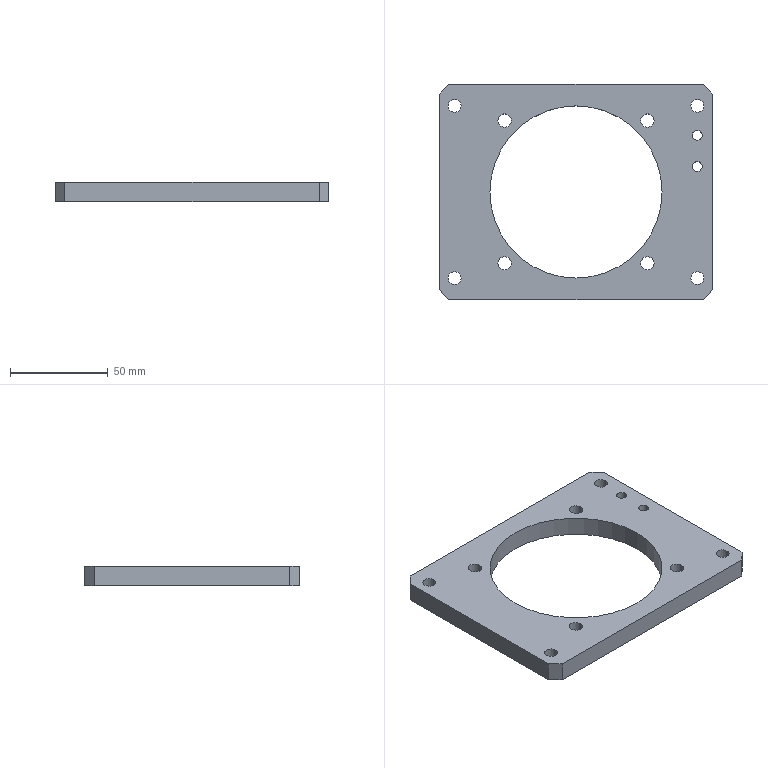Part | SolidWorks | features HoleWzd 2, Chamfer 1, Extrusion 1 | 1 solid | 32 faces | box 140 x 110 x 10 mm | volume 89465 mm3 | cylinder 22 | plane 10 | commonest cylinder face diameters 6.6 x8 6.8 x8 5 x4 88 x2
STEP:
#1=CARTESIAN_POINT('',(65.035,45.511,0.));
#2=VERTEX_POINT('',#1);
#3=CARTESIAN_POINT('',(70.035,45.511,0.));
#4=VERTEX_POINT('',#3);
#5=CARTESIAN_POINT('',(67.535,45.511,0.));
#6=DIRECTION('',(0.,0.,1.));
#7=DIRECTION('',(1.,0.,0.));
#8=AXIS2_PLACEMENT_3D('',#5,#6,#7);
#9=CIRCLE('',#8,2.5);
#10=EDGE_CURVE('',#2,#4,#9,.T.);
#11=ORIENTED_EDGE('',*,*,#10,.F.);
#12=CARTESIAN_POINT('',(65.035,45.511,10.));
#13=VERTEX_POINT('',#12);
#14=CARTESIAN_POINT('',(65.035,45.511,10.));
#15=DIRECTION('',(0.,0.,1.));
#16=VECTOR('',#15,1000.);
#17=LINE('',#14,#16);
#18=EDGE_CURVE('',#2,#13,#17,.T.);
#19=ORIENTED_EDGE('',*,*,#18,.T.);
#20=CARTESIAN_POINT('',(70.035,45.511,10.));
#21=VERTEX_POINT('',#20);
#22=CARTESIAN_POINT('',(67.535,45.511,10.));
#23=DIRECTION('',(0.,0.,1.));
#24=DIRECTION('',(1.,0.,0.));
#25=AXIS2_PLACEMENT_3D('',#22,#23,#24);
#26=CIRCLE('',#25,2.5);
#27=EDGE_CURVE('',#13,#21,#26,.T.);
#28=ORIENTED_EDGE('',*,*,#27,.T.);
#29=CARTESIAN_POINT('',(70.035,45.511,10.));
#30=DIRECTION('',(0.,0.,1.));
#31=VECTOR('',#30,1000.);
#32=LINE('',#29,#31);
#33=EDGE_CURVE('',#4,#21,#32,.T.);
#34=ORIENTED_EDGE('',*,*,#33,.F.);
#35=EDGE_LOOP('',(#11,#19,#28,#34));
#36=FACE_OUTER_BOUND('',#35,.T.);
#37=CARTESIAN_POINT('',(67.535,45.511,10.));
#38=DIRECTION('',(0.,0.,1.));
#39=DIRECTION('',(1.,0.,0.));
#40=AXIS2_PLACEMENT_3D('',#37,#38,#39);
#41=CYLINDRICAL_SURFACE('',#40,2.5);
#42=ADVANCED_FACE('',(#36),#41,.F.);
#43=CARTESIAN_POINT('',(65.035,29.511,0.));
#44=VERTEX_POINT('',#43);
#45=CARTESIAN_POINT('',(70.035,29.511,0.));
#46=VERTEX_POINT('',#45);
#47=CARTESIAN_POINT('',(67.535,29.511,0.));
#48=DIRECTION('',(0.,0.,1.));
#49=DIRECTION('',(1.,0.,0.));
#50=AXIS2_PLACEMENT_3D('',#47,#48,#49);
#51=CIRCLE('',#50,2.5);
#52=EDGE_CURVE('',#44,#46,#51,.T.);
#53=ORIENTED_EDGE('',*,*,#52,.F.);
#54=CARTESIAN_POINT('',(65.035,29.511,10.));
#55=VERTEX_POINT('',#54);
#56=CARTESIAN_POINT('',(65.035,29.511,10.));
#57=DIRECTION('',(0.,0.,1.));
#58=VECTOR('',#57,1000.);
#59=LINE('',#56,#58);
#60=EDGE_CURVE('',#44,#55,#59,.T.);
#61=ORIENTED_EDGE('',*,*,#60,.T.);
#62=CARTESIAN_POINT('',(70.035,29.511,10.));
#63=VERTEX_POINT('',#62);
#64=CARTESIAN_POINT('',(67.535,29.511,10.));
#65=DIRECTION('',(0.,0.,1.));
#66=DIRECTION('',(1.,0.,0.));
#67=AXIS2_PLACEMENT_3D('',#64,#65,#66);
#68=CIRCLE('',#67,2.5);
#69=EDGE_CURVE('',#55,#63,#68,.T.);
#70=ORIENTED_EDGE('',*,*,#69,.T.);
#71=CARTESIAN_POINT('',(70.035,29.511,10.));
#72=DIRECTION('',(0.,0.,1.));
#73=VECTOR('',#72,1000.);
#74=LINE('',#71,#73);
#75=EDGE_CURVE('',#46,#63,#74,.T.);
#76=ORIENTED_EDGE('',*,*,#75,.F.);
#77=EDGE_LOOP('',(#53,#61,#70,#76));
#78=FACE_OUTER_BOUND('',#77,.T.);
#79=CARTESIAN_POINT('',(67.535,29.511,10.));
#80=DIRECTION('',(0.,0.,1.));
#81=DIRECTION('',(1.,0.,0.));
#82=AXIS2_PLACEMENT_3D('',#79,#80,#81);
#83=CYLINDRICAL_SURFACE('',#82,2.5);
#84=ADVANCED_FACE('',(#78),#83,.F.);
#85=CARTESIAN_POINT('',(-34.365,53.011,0.));
#86=VERTEX_POINT('',#85);
#87=CARTESIAN_POINT('',(-27.565,53.011,0.));
#88=VERTEX_POINT('',#87);
#89=CARTESIAN_POINT('',(-30.965,53.011,0.));
#90=DIRECTION('',(0.,0.,1.));
#91=DIRECTION('',(1.,0.,0.));
#92=AXIS2_PLACEMENT_3D('',#89,#90,#91);
#93=CIRCLE('',#92,3.4);
#94=EDGE_CURVE('',#86,#88,#93,.T.);
#95=ORIENTED_EDGE('',*,*,#94,.F.);
#96=CARTESIAN_POINT('',(-34.365,53.011,10.));
#97=VERTEX_POINT('',#96);
#98=CARTESIAN_POINT('',(-34.365,53.011,10.));
#99=DIRECTION('',(0.,0.,1.));
#100=VECTOR('',#99,1000.);
#101=LINE('',#98,#100);
#102=EDGE_CURVE('',#86,#97,#101,.T.);
#103=ORIENTED_EDGE('',*,*,#102,.T.);
#104=CARTESIAN_POINT('',(-27.565,53.011,10.));
#105=VERTEX_POINT('',#104);
#106=CARTESIAN_POINT('',(-30.965,53.011,10.));
#107=DIRECTION('',(0.,0.,1.));
#108=DIRECTION('',(1.,0.,0.));
#109=AXIS2_PLACEMENT_3D('',#106,#107,#108);
#110=CIRCLE('',#109,3.4);
#111=EDGE_CURVE('',#97,#105,#110,.T.);
#112=ORIENTED_EDGE('',*,*,#111,.T.);
#113=CARTESIAN_POINT('',(-27.565,53.011,10.));
#114=DIRECTION('',(0.,0.,1.));
#115=VECTOR('',#114,1000.);
#116=LINE('',#113,#115);
#117=EDGE_CURVE('',#88,#105,#116,.T.);
#118=ORIENTED_EDGE('',*,*,#117,.F.);
#119=EDGE_LOOP('',(#95,#103,#112,#118));
#120=FACE_OUTER_BOUND('',#119,.T.);
#121=CARTESIAN_POINT('',(-30.965,53.011,10.));
#122=DIRECTION('',(0.,0.,1.));
#123=DIRECTION('',(1.,0.,0.));
#124=AXIS2_PLACEMENT_3D('',#121,#122,#123);
#125=CYLINDRICAL_SURFACE('',#124,3.4);
#126=ADVANCED_FACE('',(#120),#125,.F.);
#127=CARTESIAN_POINT('',(38.635,53.011,0.));
#128=VERTEX_POINT('',#127);
#129=CARTESIAN_POINT('',(45.435,53.011,0.));
#130=VERTEX_POINT('',#129);
#131=CARTESIAN_POINT('',(42.035,53.011,0.));
#132=DIRECTION('',(0.,0.,1.));
#133=DIRECTION('',(1.,0.,0.));
#134=AXIS2_PLACEMENT_3D('',#131,#132,#133);
#135=CIRCLE('',#134,3.4);
#136=EDGE_CURVE('',#128,#130,#135,.T.);
#137=ORIENTED_EDGE('',*,*,#136,.F.);
#138=CARTESIAN_POINT('',(38.635,53.011,10.));
#139=VERTEX_POINT('',#138);
#140=CARTESIAN_POINT('',(38.635,53.011,10.));
#141=DIRECTION('',(0.,0.,1.));
#142=VECTOR('',#141,1000.);
#143=LINE('',#140,#142);
#144=EDGE_CURVE('',#128,#139,#143,.T.);
#145=ORIENTED_EDGE('',*,*,#144,.T.);
#146=CARTESIAN_POINT('',(45.435,53.011,10.));
#147=VERTEX_POINT('',#146);
#148=CARTESIAN_POINT('',(42.035,53.011,10.));
#149=DIRECTION('',(0.,0.,1.));
#150=DIRECTION('',(1.,0.,0.));
#151=AXIS2_PLACEMENT_3D('',#148,#149,#150);
#152=CIRCLE('',#151,3.4);
#153=EDGE_CURVE('',#139,#147,#152,.T.);
#154=ORIENTED_EDGE('',*,*,#153,.T.);
#155=CARTESIAN_POINT('',(45.435,53.011,10.));
#156=DIRECTION('',(0.,0.,1.));
#157=VECTOR('',#156,1000.);
#158=LINE('',#155,#157);
#159=EDGE_CURVE('',#130,#147,#158,.T.);
#160=ORIENTED_EDGE('',*,*,#159,.F.);
#161=EDGE_LOOP('',(#137,#145,#154,#160));
#162=FACE_OUTER_BOUND('',#161,.T.);
#163=CARTESIAN_POINT('',(42.035,53.011,10.));
#164=DIRECTION('',(0.,0.,1.));
#165=DIRECTION('',(1.,0.,0.));
#166=AXIS2_PLACEMENT_3D('',#163,#164,#165);
#167=CYLINDRICAL_SURFACE('',#166,3.4);
#168=ADVANCED_FACE('',(#162),#167,.F.);
#169=CARTESIAN_POINT('',(38.635,-19.989,0.));
#170=VERTEX_POINT('',#169);
#171=CARTESIAN_POINT('',(45.435,-19.989,0.));
#172=VERTEX_POINT('',#171);
#173=CARTESIAN_POINT('',(42.035,-19.989,0.));
#174=DIRECTION('',(0.,0.,1.));
#175=DIRECTION('',(1.,0.,0.));
#176=AXIS2_PLACEMENT_3D('',#173,#174,#175);
#177=CIRCLE('',#176,3.4);
#178=EDGE_CURVE('',#170,#172,#177,.T.);
#179=ORIENTED_EDGE('',*,*,#178,.F.);
#180=CARTESIAN_POINT('',(38.635,-19.989,10.));
#181=VERTEX_POINT('',#180);
#182=CARTESIAN_POINT('',(38.635,-19.989,10.));
#183=DIRECTION('',(0.,0.,1.));
#184=VECTOR('',#183,1000.);
#185=LINE('',#182,#184);
#186=EDGE_CURVE('',#170,#181,#185,.T.);
#187=ORIENTED_EDGE('',*,*,#186,.T.);
#188=CARTESIAN_POINT('',(45.435,-19.989,10.));
#189=VERTEX_POINT('',#188);
#190=CARTESIAN_POINT('',(42.035,-19.989,10.));
#191=DIRECTION('',(0.,0.,1.));
#192=DIRECTION('',(1.,0.,0.));
#193=AXIS2_PLACEMENT_3D('',#190,#191,#192);
#194=CIRCLE('',#193,3.4);
#195=EDGE_CURVE('',#181,#189,#194,.T.);
#196=ORIENTED_EDGE('',*,*,#195,.T.);
#197=CARTESIAN_POINT('',(45.435,-19.989,10.));
#198=DIRECTION('',(0.,0.,1.));
#199=VECTOR('',#198,1000.);
#200=LINE('',#197,#199);
#201=EDGE_CURVE('',#172,#189,#200,.T.);
#202=ORIENTED_EDGE('',*,*,#201,.F.);
#203=EDGE_LOOP('',(#179,#187,#196,#202));
#204=FACE_OUTER_BOUND('',#203,.T.);
#205=CARTESIAN_POINT('',(42.035,-19.989,10.));
#206=DIRECTION('',(0.,0.,1.));
#207=DIRECTION('',(1.,0.,0.));
#208=AXIS2_PLACEMENT_3D('',#205,#206,#207);
#209=CYLINDRICAL_SURFACE('',#208,3.4);
#210=ADVANCED_FACE('',(#204),#209,.F.);
#211=CARTESIAN_POINT('',(-34.365,-19.989,0.));
#212=VERTEX_POINT('',#211);
#213=CARTESIAN_POINT('',(-27.565,-19.989,0.));
#214=VERTEX_POINT('',#213);
#215=CARTESIAN_POINT('',(-30.965,-19.989,0.));
#216=DIRECTION('',(0.,0.,1.));
#217=DIRECTION('',(1.,0.,0.));
#218=AXIS2_PLACEMENT_3D('',#215,#216,#217);
#219=CIRCLE('',#218,3.4);
#220=EDGE_CURVE('',#212,#214,#219,.T.);
#221=ORIENTED_EDGE('',*,*,#220,.F.);
#222=CARTESIAN_POINT('',(-34.365,-19.989,10.));
#223=VERTEX_POINT('',#222);
#224=CARTESIAN_POINT('',(-34.365,-19.989,10.));
#225=DIRECTION('',(0.,0.,1.));
#226=VECTOR('',#225,1000.);
#227=LINE('',#224,#226);
#228=EDGE_CURVE('',#212,#223,#227,.T.);
#229=ORIENTED_EDGE('',*,*,#228,.T.);
#230=CARTESIAN_POINT('',(-27.565,-19.989,10.));
#231=VERTEX_POINT('',#230);
#232=CARTESIAN_POINT('',(-30.965,-19.989,10.));
#233=DIRECTION('',(0.,0.,1.));
#234=DIRECTION('',(1.,0.,0.));
#235=AXIS2_PLACEMENT_3D('',#232,#233,#234);
#236=CIRCLE('',#235,3.4);
#237=EDGE_CURVE('',#223,#231,#236,.T.);
#238=ORIENTED_EDGE('',*,*,#237,.T.);
#239=CARTESIAN_POINT('',(-27.565,-19.989,10.));
#240=DIRECTION('',(0.,0.,1.));
#241=VECTOR('',#240,1000.);
#242=LINE('',#239,#241);
#243=EDGE_CURVE('',#214,#231,#242,.T.);
#244=ORIENTED_EDGE('',*,*,#243,.F.);
#245=EDGE_LOOP('',(#221,#229,#238,#244));
#246=FACE_OUTER_BOUND('',#245,.T.);
#247=CARTESIAN_POINT('',(-30.965,-19.989,10.));
#248=DIRECTION('',(0.,0.,1.));
#249=DIRECTION('',(1.,0.,0.));
#250=AXIS2_PLACEMENT_3D('',#247,#248,#249);
#251=CYLINDRICAL_SURFACE('',#250,3.4);
#252=ADVANCED_FACE('',(#246),#251,.F.);
#253=CARTESIAN_POINT('',(64.235,60.511,10.));
#254=VERTEX_POINT('',#253);
#255=CARTESIAN_POINT('',(70.835,60.511,10.));
#256=VERTEX_POINT('',#255);
#257=CARTESIAN_POINT('',(67.535,60.511,10.));
#258=DIRECTION('',(0.,0.,1.));
#259=DIRECTION('',(1.,0.,0.));
#260=AXIS2_PLACEMENT_3D('',#257,#258,#259);
#261=CIRCLE('',#260,3.3);
#262=EDGE_CURVE('',#254,#256,#261,.T.);
#263=ORIENTED_EDGE('',*,*,#262,.T.);
#264=CARTESIAN_POINT('',(70.835,60.511,0.));
#265=VERTEX_POINT('',#264);
#266=CARTESIAN_POINT('',(70.835,60.511,10.));
#267=DIRECTION('',(0.,0.,-1.));
#268=VECTOR('',#267,1000.);
#269=LINE('',#266,#268);
#270=EDGE_CURVE('',#256,#265,#269,.T.);
#271=ORIENTED_EDGE('',*,*,#270,.T.);
#272=CARTESIAN_POINT('',(64.235,60.511,0.));
#273=VERTEX_POINT('',#272);
#274=CARTESIAN_POINT('',(67.535,60.511,0.));
#275=DIRECTION('',(0.,0.,1.));
#276=DIRECTION('',(1.,0.,0.));
#277=AXIS2_PLACEMENT_3D('',#274,#275,#276);
#278=CIRCLE('',#277,3.3);
#279=EDGE_CURVE('',#273,#265,#278,.T.);
#280=ORIENTED_EDGE('',*,*,#279,.F.);
#281=CARTESIAN_POINT('',(64.235,60.511,10.));
#282=DIRECTION('',(0.,0.,-1.));
#283=VECTOR('',#282,1000.);
#284=LINE('',#281,#283);
#285=EDGE_CURVE('',#254,#273,#284,.T.);
#286=ORIENTED_EDGE('',*,*,#285,.F.);
#287=EDGE_LOOP('',(#263,#271,#280,#286));
#288=FACE_OUTER_BOUND('',#287,.T.);
#289=CARTESIAN_POINT('',(67.535,60.511,10.));
#290=DIRECTION('',(0.,0.,-1.));
#291=DIRECTION('',(-1.,0.,0.));
#292=AXIS2_PLACEMENT_3D('',#289,#290,#291);
#293=CYLINDRICAL_SURFACE('',#292,3.3);
#294=ADVANCED_FACE('',(#288),#293,.F.);
#295=CARTESIAN_POINT('',(64.235,-27.489,10.));
#296=VERTEX_POINT('',#295);
#297=CARTESIAN_POINT('',(70.835,-27.489,10.));
#298=VERTEX_POINT('',#297);
#299=CARTESIAN_POINT('',(67.535,-27.489,10.));
#300=DIRECTION('',(0.,0.,1.));
#301=DIRECTION('',(1.,0.,0.));
#302=AXIS2_PLACEMENT_3D('',#299,#300,#301);
#303=CIRCLE('',#302,3.3);
#304=EDGE_CURVE('',#296,#298,#303,.T.);
#305=ORIENTED_EDGE('',*,*,#304,.T.);
#306=CARTESIAN_POINT('',(70.835,-27.489,0.));
#307=VERTEX_POINT('',#306);
#308=CARTESIAN_POINT('',(70.835,-27.489,10.));
#309=DIRECTION('',(0.,0.,-1.));
#310=VECTOR('',#309,1000.);
#311=LINE('',#308,#310);
#312=EDGE_CURVE('',#298,#307,#311,.T.);
#313=ORIENTED_EDGE('',*,*,#312,.T.);
#314=CARTESIAN_POINT('',(64.235,-27.489,0.));
#315=VERTEX_POINT('',#314);
#316=CARTESIAN_POINT('',(67.535,-27.489,0.));
#317=DIRECTION('',(0.,0.,1.));
#318=DIRECTION('',(1.,0.,0.));
#319=AXIS2_PLACEMENT_3D('',#316,#317,#318);
#320=CIRCLE('',#319,3.3);
#321=EDGE_CURVE('',#315,#307,#320,.T.);
#322=ORIENTED_EDGE('',*,*,#321,.F.);
#323=CARTESIAN_POINT('',(64.235,-27.489,10.));
#324=DIRECTION('',(0.,0.,-1.));
#325=VECTOR('',#324,1000.);
#326=LINE('',#323,#325);
#327=EDGE_CURVE('',#296,#315,#326,.T.);
#328=ORIENTED_EDGE('',*,*,#327,.F.);
#329=EDGE_LOOP('',(#305,#313,#322,#328));
#330=FACE_OUTER_BOUND('',#329,.T.);
#331=CARTESIAN_POINT('',(67.535,-27.489,10.));
#332=DIRECTION('',(0.,0.,-1.));
#333=DIRECTION('',(-1.,0.,0.));
#334=AXIS2_PLACEMENT_3D('',#331,#332,#333);
#335=CYLINDRICAL_SURFACE('',#334,3.3);
#336=ADVANCED_FACE('',(#330),#335,.F.);
#337=CARTESIAN_POINT('',(-59.765,-27.489,10.));
#338=VERTEX_POINT('',#337);
#339=CARTESIAN_POINT('',(-53.165,-27.489,10.));
#340=VERTEX_POINT('',#339);
#341=CARTESIAN_POINT('',(-56.465,-27.489,10.));
#342=DIRECTION('',(0.,0.,1.));
#343=DIRECTION('',(1.,0.,0.));
#344=AXIS2_PLACEMENT_3D('',#341,#342,#343);
#345=CIRCLE('',#344,3.3);
#346=EDGE_CURVE('',#338,#340,#345,.T.);
#347=ORIENTED_EDGE('',*,*,#346,.T.);
#348=CARTESIAN_POINT('',(-53.165,-27.489,0.));
#349=VERTEX_POINT('',#348);
#350=CARTESIAN_POINT('',(-53.165,-27.489,10.));
#351=DIRECTION('',(0.,0.,-1.));
#352=VECTOR('',#351,1000.);
#353=LINE('',#350,#352);
#354=EDGE_CURVE('',#340,#349,#353,.T.);
#355=ORIENTED_EDGE('',*,*,#354,.T.);
#356=CARTESIAN_POINT('',(-59.765,-27.489,0.));
#357=VERTEX_POINT('',#356);
#358=CARTESIAN_POINT('',(-56.465,-27.489,0.));
#359=DIRECTION('',(0.,0.,1.));
#360=DIRECTION('',(1.,0.,0.));
#361=AXIS2_PLACEMENT_3D('',#358,#359,#360);
#362=CIRCLE('',#361,3.3);
#363=EDGE_CURVE('',#357,#349,#362,.T.);
#364=ORIENTED_EDGE('',*,*,#363,.F.);
#365=CARTESIAN_POINT('',(-59.765,-27.489,10.));
#366=DIRECTION('',(0.,0.,-1.));
#367=VECTOR('',#366,1000.);
#368=LINE('',#365,#367);
#369=EDGE_CURVE('',#338,#357,#368,.T.);
#370=ORIENTED_EDGE('',*,*,#369,.F.);
#371=EDGE_LOOP('',(#347,#355,#364,#370));
#372=FACE_OUTER_BOUND('',#371,.T.);
#373=CARTESIAN_POINT('',(-56.465,-27.489,10.));
#374=DIRECTION('',(0.,0.,-1.));
#375=DIRECTION('',(-1.,0.,0.));
#376=AXIS2_PLACEMENT_3D('',#373,#374,#375);
#377=CYLINDRICAL_SURFACE('',#376,3.3);
#378=ADVANCED_FACE('',(#372),#377,.F.);
#379=CARTESIAN_POINT('',(-59.765,60.511,10.));
#380=VERTEX_POINT('',#379);
#381=CARTESIAN_POINT('',(-53.165,60.511,10.));
#382=VERTEX_POINT('',#381);
#383=CARTESIAN_POINT('',(-56.465,60.511,10.));
#384=DIRECTION('',(0.,0.,1.));
#385=DIRECTION('',(1.,0.,0.));
#386=AXIS2_PLACEMENT_3D('',#383,#384,#385);
#387=CIRCLE('',#386,3.3);
#388=EDGE_CURVE('',#380,#382,#387,.T.);
#389=ORIENTED_EDGE('',*,*,#388,.T.);
#390=CARTESIAN_POINT('',(-53.165,60.511,0.));
#391=VERTEX_POINT('',#390);
#392=CARTESIAN_POINT('',(-53.165,60.511,10.));
#393=DIRECTION('',(0.,0.,-1.));
#394=VECTOR('',#393,1000.);
#395=LINE('',#392,#394);
#396=EDGE_CURVE('',#382,#391,#395,.T.);
#397=ORIENTED_EDGE('',*,*,#396,.T.);
#398=CARTESIAN_POINT('',(-59.765,60.511,0.));
#399=VERTEX_POINT('',#398);
#400=CARTESIAN_POINT('',(-56.465,60.511,0.));
#401=DIRECTION('',(0.,0.,1.));
#402=DIRECTION('',(1.,0.,0.));
#403=AXIS2_PLACEMENT_3D('',#400,#401,#402);
#404=CIRCLE('',#403,3.3);
#405=EDGE_CURVE('',#399,#391,#404,.T.);
#406=ORIENTED_EDGE('',*,*,#405,.F.);
#407=CARTESIAN_POINT('',(-59.765,60.511,10.));
#408=DIRECTION('',(0.,0.,-1.));
#409=VECTOR('',#408,1000.);
#410=LINE('',#407,#409);
#411=EDGE_CURVE('',#380,#399,#410,.T.);
#412=ORIENTED_EDGE('',*,*,#411,.F.);
#413=EDGE_LOOP('',(#389,#397,#406,#412));
#414=FACE_OUTER_BOUND('',#413,.T.);
#415=CARTESIAN_POINT('',(-56.465,60.511,10.));
#416=DIRECTION('',(0.,0.,-1.));
#417=DIRECTION('',(-1.,0.,0.));
#418=AXIS2_PLACEMENT_3D('',#415,#416,#417);
#419=CYLINDRICAL_SURFACE('',#418,3.3);
#420=ADVANCED_FACE('',(#414),#419,.F.);
#421=CARTESIAN_POINT('',(-38.465,16.511,10.));
#422=VERTEX_POINT('',#421);
#423=CARTESIAN_POINT('',(49.535,16.511,10.));
#424=VERTEX_POINT('',#423);
#425=CARTESIAN_POINT('',(5.535,16.511,10.));
#426=DIRECTION('',(0.,0.,1.));
#427=DIRECTION('',(1.,0.,0.));
#428=AXIS2_PLACEMENT_3D('',#425,#426,#427);
#429=CIRCLE('',#428,44.);
#430=EDGE_CURVE('',#422,#424,#429,.T.);
#431=ORIENTED_EDGE('',*,*,#430,.T.);
#432=CARTESIAN_POINT('',(49.535,16.511,0.));
#433=VERTEX_POINT('',#432);
#434=CARTESIAN_POINT('',(49.535,16.511,10.));
#435=DIRECTION('',(0.,0.,-1.));
#436=VECTOR('',#435,1000.);
#437=LINE('',#434,#436);
#438=EDGE_CURVE('',#424,#433,#437,.T.);
#439=ORIENTED_EDGE('',*,*,#438,.T.);
#440=CARTESIAN_POINT('',(-38.465,16.511,0.));
#441=VERTEX_POINT('',#440);
#442=CARTESIAN_POINT('',(5.535,16.511,0.));
#443=DIRECTION('',(0.,0.,1.));
#444=DIRECTION('',(1.,0.,0.));
#445=AXIS2_PLACEMENT_3D('',#442,#443,#444);
#446=CIRCLE('',#445,44.);
#447=EDGE_CURVE('',#441,#433,#446,.T.);
#448=ORIENTED_EDGE('',*,*,#447,.F.);
#449=CARTESIAN_POINT('',(-38.465,16.511,10.));
#450=DIRECTION('',(0.,0.,-1.));
#451=VECTOR('',#450,1000.);
#452=LINE('',#449,#451);
#453=EDGE_CURVE('',#422,#441,#452,.T.);
#454=ORIENTED_EDGE('',*,*,#453,.F.);
#455=EDGE_LOOP('',(#431,#439,#448,#454));
#456=FACE_OUTER_BOUND('',#455,.T.);
#457=CARTESIAN_POINT('',(5.535,16.511,10.));
#458=DIRECTION('',(0.,0.,-1.));
#459=DIRECTION('',(-1.,0.,0.));
#460=AXIS2_PLACEMENT_3D('',#457,#458,#459);
#461=CYLINDRICAL_SURFACE('',#460,44.);
#462=ADVANCED_FACE('',(#456),#461,.F.);
#463=CARTESIAN_POINT('',(75.535,66.511,10.));
#464=VERTEX_POINT('',#463);
#465=CARTESIAN_POINT('',(75.535,-33.489,10.));
#466=VERTEX_POINT('',#465);
#467=CARTESIAN_POINT('',(75.535,0.,10.));
#468=DIRECTION('',(0.,-1.,0.));
#469=VECTOR('',#468,1000.);
#470=LINE('',#467,#469);
#471=EDGE_CURVE('',#464,#466,#470,.T.);
#472=ORIENTED_EDGE('',*,*,#471,.T.);
#473=CARTESIAN_POINT('',(75.535,-33.489,0.));
#474=VERTEX_POINT('',#473);
#475=CARTESIAN_POINT('',(75.535,-33.489,0.));
#476=DIRECTION('',(0.,0.,-1.));
#477=VECTOR('',#476,1000.);
#478=LINE('',#475,#477);
#479=EDGE_CURVE('',#466,#474,#478,.T.);
#480=ORIENTED_EDGE('',*,*,#479,.T.);
#481=CARTESIAN_POINT('',(75.535,66.511,0.));
#482=VERTEX_POINT('',#481);
#483=CARTESIAN_POINT('',(75.535,0.,0.));
#484=DIRECTION('',(0.,-1.,0.));
#485=VECTOR('',#484,1000.);
#486=LINE('',#483,#485);
#487=EDGE_CURVE('',#482,#474,#486,.T.);
#488=ORIENTED_EDGE('',*,*,#487,.F.);
#489=CARTESIAN_POINT('',(75.535,66.511,10.));
#490=DIRECTION('',(0.,0.,1.));
#491=VECTOR('',#490,1000.);
#492=LINE('',#489,#491);
#493=EDGE_CURVE('',#482,#464,#492,.T.);
#494=ORIENTED_EDGE('',*,*,#493,.T.);
#495=EDGE_LOOP('',(#472,#480,#488,#494));
#496=FACE_OUTER_BOUND('',#495,.T.);
#497=CARTESIAN_POINT('',(75.535,0.,10.));
#498=DIRECTION('',(1.,0.,0.));
#499=DIRECTION('',(0.,1.,0.));
#500=AXIS2_PLACEMENT_3D('',#497,#498,#499);
#501=PLANE('',#500);
#502=ADVANCED_FACE('',(#496),#501,.T.);
#503=CARTESIAN_POINT('',(-59.465,71.511,10.));
#504=VERTEX_POINT('',#503);
#505=CARTESIAN_POINT('',(70.535,71.511,10.));
#506=VERTEX_POINT('',#505);
#507=CARTESIAN_POINT('',(0.,71.511,10.));
#508=DIRECTION('',(1.,0.,0.));
#509=VECTOR('',#508,1000.);
#510=LINE('',#507,#509);
#511=EDGE_CURVE('',#504,#506,#510,.T.);
#512=ORIENTED_EDGE('',*,*,#511,.T.);
#513=CARTESIAN_POINT('',(70.535,71.511,0.));
#514=VERTEX_POINT('',#513);
#515=CARTESIAN_POINT('',(70.535,71.511,10.));
#516=DIRECTION('',(0.,0.,-1.));
#517=VECTOR('',#516,1000.);
#518=LINE('',#515,#517);
#519=EDGE_CURVE('',#506,#514,#518,.T.);
#520=ORIENTED_EDGE('',*,*,#519,.T.);
#521=CARTESIAN_POINT('',(-59.465,71.511,0.));
#522=VERTEX_POINT('',#521);
#523=CARTESIAN_POINT('',(0.,71.511,0.));
#524=DIRECTION('',(1.,0.,0.));
#525=VECTOR('',#524,1000.);
#526=LINE('',#523,#525);
#527=EDGE_CURVE('',#522,#514,#526,.T.);
#528=ORIENTED_EDGE('',*,*,#527,.F.);
#529=CARTESIAN_POINT('',(-59.465,71.511,10.));
#530=DIRECTION('',(0.,0.,1.));
#531=VECTOR('',#530,1000.);
#532=LINE('',#529,#531);
#533=EDGE_CURVE('',#522,#504,#532,.T.);
#534=ORIENTED_EDGE('',*,*,#533,.T.);
#535=EDGE_LOOP('',(#512,#520,#528,#534));
#536=FACE_OUTER_BOUND('',#535,.T.);
#537=CARTESIAN_POINT('',(0.,71.511,10.));
#538=DIRECTION('',(0.,1.,0.));
#539=DIRECTION('',(0.,0.,1.));
#540=AXIS2_PLACEMENT_3D('',#537,#538,#539);
#541=PLANE('',#540);
#542=ADVANCED_FACE('',(#536),#541,.T.);
#543=CARTESIAN_POINT('',(-64.465,66.511,10.));
#544=VERTEX_POINT('',#543);
#545=CARTESIAN_POINT('',(-64.465,-33.489,10.));
#546=VERTEX_POINT('',#545);
#547=CARTESIAN_POINT('',(-64.465,0.,10.));
#548=DIRECTION('',(0.,-1.,0.));
#549=VECTOR('',#548,1000.);
#550=LINE('',#547,#549);
#551=EDGE_CURVE('',#544,#546,#550,.T.);
#552=ORIENTED_EDGE('',*,*,#551,.F.);
#553=CARTESIAN_POINT('',(-64.465,66.511,0.));
#554=VERTEX_POINT('',#553);
#555=CARTESIAN_POINT('',(-64.465,66.511,0.));
#556=DIRECTION('',(0.,0.,-1.));
#557=VECTOR('',#556,1000.);
#558=LINE('',#555,#557);
#559=EDGE_CURVE('',#544,#554,#558,.T.);
#560=ORIENTED_EDGE('',*,*,#559,.T.);
#561=CARTESIAN_POINT('',(-64.465,-33.489,0.));
#562=VERTEX_POINT('',#561);
#563=CARTESIAN_POINT('',(-64.465,0.,0.));
#564=DIRECTION('',(0.,-1.,0.));
#565=VECTOR('',#564,1000.);
#566=LINE('',#563,#565);
#567=EDGE_CURVE('',#554,#562,#566,.T.);
#568=ORIENTED_EDGE('',*,*,#567,.T.);
#569=CARTESIAN_POINT('',(-64.465,-33.489,10.));
#570=DIRECTION('',(0.,0.,1.));
#571=VECTOR('',#570,1000.);
#572=LINE('',#569,#571);
#573=EDGE_CURVE('',#562,#546,#572,.T.);
#574=ORIENTED_EDGE('',*,*,#573,.T.);
#575=EDGE_LOOP('',(#552,#560,#568,#574));
#576=FACE_OUTER_BOUND('',#575,.T.);
#577=CARTESIAN_POINT('',(-64.465,0.,10.));
#578=DIRECTION('',(1.,0.,0.));
#579=DIRECTION('',(0.,0.,-1.));
#580=AXIS2_PLACEMENT_3D('',#577,#578,#579);
#581=PLANE('',#580);
#582=ADVANCED_FACE('',(#576),#581,.F.);
#583=ORIENTED_EDGE('',*,*,#438,.F.);
#584=CARTESIAN_POINT('',(5.535,16.511,10.));
#585=DIRECTION('',(0.,0.,1.));
#586=DIRECTION('',(1.,0.,0.));
#587=AXIS2_PLACEMENT_3D('',#584,#585,#586);
#588=CIRCLE('',#587,44.);
#589=EDGE_CURVE('',#424,#422,#588,.T.);
#590=ORIENTED_EDGE('',*,*,#589,.T.);
#591=ORIENTED_EDGE('',*,*,#453,.T.);
#592=CARTESIAN_POINT('',(5.535,16.511,0.));
#593=DIRECTION('',(0.,0.,1.));
#594=DIRECTION('',(1.,0.,0.));
#595=AXIS2_PLACEMENT_3D('',#592,#593,#594);
#596=CIRCLE('',#595,44.);
#597=EDGE_CURVE('',#433,#441,#596,.T.);
#598=ORIENTED_EDGE('',*,*,#597,.F.);
#599=EDGE_LOOP('',(#583,#590,#591,#598));
#600=FACE_OUTER_BOUND('',#599,.T.);
#601=CARTESIAN_POINT('',(5.535,16.511,10.));
#602=DIRECTION('',(0.,0.,-1.));
#603=DIRECTION('',(-1.,0.,0.));
#604=AXIS2_PLACEMENT_3D('',#601,#602,#603);
#605=CYLINDRICAL_SURFACE('',#604,44.);
#606=ADVANCED_FACE('',(#600),#605,.F.);
#607=ORIENTED_EDGE('',*,*,#396,.F.);
#608=CARTESIAN_POINT('',(-56.465,60.511,10.));
#609=DIRECTION('',(0.,0.,1.));
#610=DIRECTION('',(1.,0.,0.));
#611=AXIS2_PLACEMENT_3D('',#608,#609,#610);
#612=CIRCLE('',#611,3.3);
#613=EDGE_CURVE('',#382,#380,#612,.T.);
#614=ORIENTED_EDGE('',*,*,#613,.T.);
#615=ORIENTED_EDGE('',*,*,#411,.T.);
#616=CARTESIAN_POINT('',(-56.465,60.511,0.));
#617=DIRECTION('',(0.,0.,1.));
#618=DIRECTION('',(1.,0.,0.));
#619=AXIS2_PLACEMENT_3D('',#616,#617,#618);
#620=CIRCLE('',#619,3.3);
#621=EDGE_CURVE('',#391,#399,#620,.T.);
#622=ORIENTED_EDGE('',*,*,#621,.F.);
#623=EDGE_LOOP('',(#607,#614,#615,#622));
#624=FACE_OUTER_BOUND('',#623,.T.);
#625=CARTESIAN_POINT('',(-56.465,60.511,10.));
#626=DIRECTION('',(0.,0.,-1.));
#627=DIRECTION('',(-1.,0.,0.));
#628=AXIS2_PLACEMENT_3D('',#625,#626,#627);
#629=CYLINDRICAL_SURFACE('',#628,3.3);
#630=ADVANCED_FACE('',(#624),#629,.F.);
#631=ORIENTED_EDGE('',*,*,#354,.F.);
#632=CARTESIAN_POINT('',(-56.465,-27.489,10.));
#633=DIRECTION('',(0.,0.,1.));
#634=DIRECTION('',(1.,0.,0.));
#635=AXIS2_PLACEMENT_3D('',#632,#633,#634);
#636=CIRCLE('',#635,3.3);
#637=EDGE_CURVE('',#340,#338,#636,.T.);
#638=ORIENTED_EDGE('',*,*,#637,.T.);
#639=ORIENTED_EDGE('',*,*,#369,.T.);
#640=CARTESIAN_POINT('',(-56.465,-27.489,0.));
#641=DIRECTION('',(0.,0.,1.));
#642=DIRECTION('',(1.,0.,0.));
#643=AXIS2_PLACEMENT_3D('',#640,#641,#642);
#644=CIRCLE('',#643,3.3);
#645=EDGE_CURVE('',#349,#357,#644,.T.);
#646=ORIENTED_EDGE('',*,*,#645,.F.);
#647=EDGE_LOOP('',(#631,#638,#639,#646));
#648=FACE_OUTER_BOUND('',#647,.T.);
#649=CARTESIAN_POINT('',(-56.465,-27.489,10.));
#650=DIRECTION('',(0.,0.,-1.));
#651=DIRECTION('',(-1.,0.,0.));
#652=AXIS2_PLACEMENT_3D('',#649,#650,#651);
#653=CYLINDRICAL_SURFACE('',#652,3.3);
#654=ADVANCED_FACE('',(#648),#653,.F.);
#655=ORIENTED_EDGE('',*,*,#312,.F.);
#656=CARTESIAN_POINT('',(67.535,-27.489,10.));
#657=DIRECTION('',(0.,0.,1.));
#658=DIRECTION('',(1.,0.,0.));
#659=AXIS2_PLACEMENT_3D('',#656,#657,#658);
#660=CIRCLE('',#659,3.3);
#661=EDGE_CURVE('',#298,#296,#660,.T.);
#662=ORIENTED_EDGE('',*,*,#661,.T.);
#663=ORIENTED_EDGE('',*,*,#327,.T.);
#664=CARTESIAN_POINT('',(67.535,-27.489,0.));
#665=DIRECTION('',(0.,0.,1.));
#666=DIRECTION('',(1.,0.,0.));
#667=AXIS2_PLACEMENT_3D('',#664,#665,#666);
#668=CIRCLE('',#667,3.3);
#669=EDGE_CURVE('',#307,#315,#668,.T.);
#670=ORIENTED_EDGE('',*,*,#669,.F.);
#671=EDGE_LOOP('',(#655,#662,#663,#670));
#672=FACE_OUTER_BOUND('',#671,.T.);
#673=CARTESIAN_POINT('',(67.535,-27.489,10.));
#674=DIRECTION('',(0.,0.,-1.));
#675=DIRECTION('',(-1.,0.,0.));
#676=AXIS2_PLACEMENT_3D('',#673,#674,#675);
#677=CYLINDRICAL_SURFACE('',#676,3.3);
#678=ADVANCED_FACE('',(#672),#677,.F.);
#679=ORIENTED_EDGE('',*,*,#270,.F.);
#680=CARTESIAN_POINT('',(67.535,60.511,10.));
#681=DIRECTION('',(0.,0.,1.));
#682=DIRECTION('',(1.,0.,0.));
#683=AXIS2_PLACEMENT_3D('',#680,#681,#682);
#684=CIRCLE('',#683,3.3);
#685=EDGE_CURVE('',#256,#254,#684,.T.);
#686=ORIENTED_EDGE('',*,*,#685,.T.);
#687=ORIENTED_EDGE('',*,*,#285,.T.);
#688=CARTESIAN_POINT('',(67.535,60.511,0.));
#689=DIRECTION('',(0.,0.,1.));
#690=DIRECTION('',(1.,0.,0.));
#691=AXIS2_PLACEMENT_3D('',#688,#689,#690);
#692=CIRCLE('',#691,3.3);
#693=EDGE_CURVE('',#265,#273,#692,.T.);
#694=ORIENTED_EDGE('',*,*,#693,.F.);
#695=EDGE_LOOP('',(#679,#686,#687,#694));
#696=FACE_OUTER_BOUND('',#695,.T.);
#697=CARTESIAN_POINT('',(67.535,60.511,10.));
#698=DIRECTION('',(0.,0.,-1.));
#699=DIRECTION('',(-1.,0.,0.));
#700=AXIS2_PLACEMENT_3D('',#697,#698,#699);
#701=CYLINDRICAL_SURFACE('',#700,3.3);
#702=ADVANCED_FACE('',(#696),#701,.F.);
#703=CARTESIAN_POINT('',(-59.465,-38.489,0.));
#704=VERTEX_POINT('',#703);
#705=CARTESIAN_POINT('',(70.535,-38.489,0.));
#706=VERTEX_POINT('',#705);
#707=CARTESIAN_POINT('',(0.,-38.489,0.));
#708=DIRECTION('',(1.,0.,0.));
#709=VECTOR('',#708,1000.);
#710=LINE('',#707,#709);
#711=EDGE_CURVE('',#704,#706,#710,.T.);
#712=ORIENTED_EDGE('',*,*,#711,.T.);
#713=CARTESIAN_POINT('',(70.535,-38.489,10.));
#714=VERTEX_POINT('',#713);
#715=CARTESIAN_POINT('',(70.535,-38.489,10.));
#716=DIRECTION('',(0.,0.,1.));
#717=VECTOR('',#716,1000.);
#718=LINE('',#715,#717);
#719=EDGE_CURVE('',#706,#714,#718,.T.);
#720=ORIENTED_EDGE('',*,*,#719,.T.);
#721=CARTESIAN_POINT('',(-59.465,-38.489,10.));
#722=VERTEX_POINT('',#721);
#723=CARTESIAN_POINT('',(0.,-38.489,10.));
#724=DIRECTION('',(1.,0.,0.));
#725=VECTOR('',#724,1000.);
#726=LINE('',#723,#725);
#727=EDGE_CURVE('',#722,#714,#726,.T.);
#728=ORIENTED_EDGE('',*,*,#727,.F.);
#729=CARTESIAN_POINT('',(-59.465,-38.489,10.));
#730=DIRECTION('',(0.,0.,-1.));
#731=VECTOR('',#730,1000.);
#732=LINE('',#729,#731);
#733=EDGE_CURVE('',#722,#704,#732,.T.);
#734=ORIENTED_EDGE('',*,*,#733,.T.);
#735=EDGE_LOOP('',(#712,#720,#728,#734));
#736=FACE_OUTER_BOUND('',#735,.T.);
#737=CARTESIAN_POINT('',(0.,-38.489,10.));
#738=DIRECTION('',(0.,1.,0.));
#739=DIRECTION('',(0.,0.,1.));
#740=AXIS2_PLACEMENT_3D('',#737,#738,#739);
#741=PLANE('',#740);
#742=ADVANCED_FACE('',(#736),#741,.F.);
#743=CARTESIAN_POINT('',(67.535,45.511,10.));
#744=DIRECTION('',(0.,0.,1.));
#745=DIRECTION('',(1.,0.,0.));
#746=AXIS2_PLACEMENT_3D('',#743,#744,#745);
#747=CIRCLE('',#746,2.5);
#748=EDGE_CURVE('',#21,#13,#747,.T.);
#749=ORIENTED_EDGE('',*,*,#748,.F.);
#750=ORIENTED_EDGE('',*,*,#27,.F.);
#751=EDGE_LOOP('',(#749,#750));
#752=FACE_BOUND('',#751,.T.);
#753=CARTESIAN_POINT('',(67.535,29.511,10.));
#754=DIRECTION('',(0.,0.,1.));
#755=DIRECTION('',(1.,0.,0.));
#756=AXIS2_PLACEMENT_3D('',#753,#754,#755);
#757=CIRCLE('',#756,2.5);
#758=EDGE_CURVE('',#63,#55,#757,.T.);
#759=ORIENTED_EDGE('',*,*,#758,.F.);
#760=ORIENTED_EDGE('',*,*,#69,.F.);
#761=EDGE_LOOP('',(#759,#760));
#762=FACE_BOUND('',#761,.T.);
#763=CARTESIAN_POINT('',(-30.965,53.011,10.));
#764=DIRECTION('',(0.,0.,1.));
#765=DIRECTION('',(1.,0.,0.));
#766=AXIS2_PLACEMENT_3D('',#763,#764,#765);
#767=CIRCLE('',#766,3.4);
#768=EDGE_CURVE('',#105,#97,#767,.T.);
#769=ORIENTED_EDGE('',*,*,#768,.F.);
#770=ORIENTED_EDGE('',*,*,#111,.F.);
#771=EDGE_LOOP('',(#769,#770));
#772=FACE_BOUND('',#771,.T.);
#773=CARTESIAN_POINT('',(42.035,53.011,10.));
#774=DIRECTION('',(0.,0.,1.));
#775=DIRECTION('',(1.,0.,0.));
#776=AXIS2_PLACEMENT_3D('',#773,#774,#775);
#777=CIRCLE('',#776,3.4);
#778=EDGE_CURVE('',#147,#139,#777,.T.);
#779=ORIENTED_EDGE('',*,*,#778,.F.);
#780=ORIENTED_EDGE('',*,*,#153,.F.);
#781=EDGE_LOOP('',(#779,#780));
#782=FACE_BOUND('',#781,.T.);
#783=CARTESIAN_POINT('',(42.035,-19.989,10.));
#784=DIRECTION('',(0.,0.,1.));
#785=DIRECTION('',(1.,0.,0.));
#786=AXIS2_PLACEMENT_3D('',#783,#784,#785);
#787=CIRCLE('',#786,3.4);
#788=EDGE_CURVE('',#189,#181,#787,.T.);
#789=ORIENTED_EDGE('',*,*,#788,.F.);
#790=ORIENTED_EDGE('',*,*,#195,.F.);
#791=EDGE_LOOP('',(#789,#790));
#792=FACE_BOUND('',#791,.T.);
#793=CARTESIAN_POINT('',(-30.965,-19.989,10.));
#794=DIRECTION('',(0.,0.,1.));
#795=DIRECTION('',(1.,0.,0.));
#796=AXIS2_PLACEMENT_3D('',#793,#794,#795);
#797=CIRCLE('',#796,3.4);
#798=EDGE_CURVE('',#231,#223,#797,.T.);
#799=ORIENTED_EDGE('',*,*,#798,.F.);
#800=ORIENTED_EDGE('',*,*,#237,.F.);
#801=EDGE_LOOP('',(#799,#800));
#802=FACE_BOUND('',#801,.T.);
#803=ORIENTED_EDGE('',*,*,#262,.F.);
#804=ORIENTED_EDGE('',*,*,#685,.F.);
#805=EDGE_LOOP('',(#803,#804));
#806=FACE_BOUND('',#805,.T.);
#807=ORIENTED_EDGE('',*,*,#304,.F.);
#808=ORIENTED_EDGE('',*,*,#661,.F.);
#809=EDGE_LOOP('',(#807,#808));
#810=FACE_BOUND('',#809,.T.);
#811=ORIENTED_EDGE('',*,*,#346,.F.);
#812=ORIENTED_EDGE('',*,*,#637,.F.);
#813=EDGE_LOOP('',(#811,#812));
#814=FACE_BOUND('',#813,.T.);
#815=ORIENTED_EDGE('',*,*,#388,.F.);
#816=ORIENTED_EDGE('',*,*,#613,.F.);
#817=EDGE_LOOP('',(#815,#816));
#818=FACE_BOUND('',#817,.T.);
#819=ORIENTED_EDGE('',*,*,#430,.F.);
#820=ORIENTED_EDGE('',*,*,#589,.F.);
#821=EDGE_LOOP('',(#819,#820));
#822=FACE_BOUND('',#821,.T.);
#823=ORIENTED_EDGE('',*,*,#727,.T.);
#824=CARTESIAN_POINT('',(54.512,-54.512,10.));
#825=DIRECTION('',(0.7071,0.7071,0.));
#826=VECTOR('',#825,1000.);
#827=LINE('',#824,#826);
#828=EDGE_CURVE('',#714,#466,#827,.T.);
#829=ORIENTED_EDGE('',*,*,#828,.T.);
#830=ORIENTED_EDGE('',*,*,#471,.F.);
#831=CARTESIAN_POINT('',(71.023,71.023,10.));
#832=DIRECTION('',(-0.7071,0.7071,0.));
#833=VECTOR('',#832,1000.);
#834=LINE('',#831,#833);
#835=EDGE_CURVE('',#464,#506,#834,.T.);
#836=ORIENTED_EDGE('',*,*,#835,.T.);
#837=ORIENTED_EDGE('',*,*,#511,.F.);
#838=CARTESIAN_POINT('',(-65.488,65.488,10.));
#839=DIRECTION('',(-0.7071,-0.7071,0.));
#840=VECTOR('',#839,1000.);
#841=LINE('',#838,#840);
#842=EDGE_CURVE('',#504,#544,#841,.T.);
#843=ORIENTED_EDGE('',*,*,#842,.T.);
#844=ORIENTED_EDGE('',*,*,#551,.T.);
#845=CARTESIAN_POINT('',(-48.977,-48.977,10.));
#846=DIRECTION('',(0.7071,-0.7071,0.));
#847=VECTOR('',#846,1000.);
#848=LINE('',#845,#847);
#849=EDGE_CURVE('',#546,#722,#848,.T.);
#850=ORIENTED_EDGE('',*,*,#849,.T.);
#851=EDGE_LOOP('',(#823,#829,#830,#836,#837,#843,#844,#850));
#852=FACE_OUTER_BOUND('',#851,.T.);
#853=CARTESIAN_POINT('',(0.,0.,10.));
#854=DIRECTION('',(0.,0.,1.));
#855=DIRECTION('',(1.,0.,0.));
#856=AXIS2_PLACEMENT_3D('',#853,#854,#855);
#857=PLANE('',#856);
#858=ADVANCED_FACE('',(#752,#762,#772,#782,#792,#802,#806,#810,#814,#818,#822,#852),#857,.T.);
#859=CARTESIAN_POINT('',(67.535,45.511,0.));
#860=DIRECTION('',(0.,0.,1.));
#861=DIRECTION('',(1.,0.,0.));
#862=AXIS2_PLACEMENT_3D('',#859,#860,#861);
#863=CIRCLE('',#862,2.5);
#864=EDGE_CURVE('',#4,#2,#863,.T.);
#865=ORIENTED_EDGE('',*,*,#864,.T.);
#866=ORIENTED_EDGE('',*,*,#10,.T.);
#867=EDGE_LOOP('',(#865,#866));
#868=FACE_BOUND('',#867,.T.);
#869=CARTESIAN_POINT('',(67.535,29.511,0.));
#870=DIRECTION('',(0.,0.,1.));
#871=DIRECTION('',(1.,0.,0.));
#872=AXIS2_PLACEMENT_3D('',#869,#870,#871);
#873=CIRCLE('',#872,2.5);
#874=EDGE_CURVE('',#46,#44,#873,.T.);
#875=ORIENTED_EDGE('',*,*,#874,.T.);
#876=ORIENTED_EDGE('',*,*,#52,.T.);
#877=EDGE_LOOP('',(#875,#876));
#878=FACE_BOUND('',#877,.T.);
#879=CARTESIAN_POINT('',(-30.965,53.011,0.));
#880=DIRECTION('',(0.,0.,1.));
#881=DIRECTION('',(1.,0.,0.));
#882=AXIS2_PLACEMENT_3D('',#879,#880,#881);
#883=CIRCLE('',#882,3.4);
#884=EDGE_CURVE('',#88,#86,#883,.T.);
#885=ORIENTED_EDGE('',*,*,#884,.T.);
#886=ORIENTED_EDGE('',*,*,#94,.T.);
#887=EDGE_LOOP('',(#885,#886));
#888=FACE_BOUND('',#887,.T.);
#889=CARTESIAN_POINT('',(42.035,53.011,0.));
#890=DIRECTION('',(0.,0.,1.));
#891=DIRECTION('',(1.,0.,0.));
#892=AXIS2_PLACEMENT_3D('',#889,#890,#891);
#893=CIRCLE('',#892,3.4);
#894=EDGE_CURVE('',#130,#128,#893,.T.);
#895=ORIENTED_EDGE('',*,*,#894,.T.);
#896=ORIENTED_EDGE('',*,*,#136,.T.);
#897=EDGE_LOOP('',(#895,#896));
#898=FACE_BOUND('',#897,.T.);
#899=CARTESIAN_POINT('',(42.035,-19.989,0.));
#900=DIRECTION('',(0.,0.,1.));
#901=DIRECTION('',(1.,0.,0.));
#902=AXIS2_PLACEMENT_3D('',#899,#900,#901);
#903=CIRCLE('',#902,3.4);
#904=EDGE_CURVE('',#172,#170,#903,.T.);
#905=ORIENTED_EDGE('',*,*,#904,.T.);
#906=ORIENTED_EDGE('',*,*,#178,.T.);
#907=EDGE_LOOP('',(#905,#906));
#908=FACE_BOUND('',#907,.T.);
#909=CARTESIAN_POINT('',(-30.965,-19.989,0.));
#910=DIRECTION('',(0.,0.,1.));
#911=DIRECTION('',(1.,0.,0.));
#912=AXIS2_PLACEMENT_3D('',#909,#910,#911);
#913=CIRCLE('',#912,3.4);
#914=EDGE_CURVE('',#214,#212,#913,.T.);
#915=ORIENTED_EDGE('',*,*,#914,.T.);
#916=ORIENTED_EDGE('',*,*,#220,.T.);
#917=EDGE_LOOP('',(#915,#916));
#918=FACE_BOUND('',#917,.T.);
#919=ORIENTED_EDGE('',*,*,#279,.T.);
#920=ORIENTED_EDGE('',*,*,#693,.T.);
#921=EDGE_LOOP('',(#919,#920));
#922=FACE_BOUND('',#921,.T.);
#923=ORIENTED_EDGE('',*,*,#321,.T.);
#924=ORIENTED_EDGE('',*,*,#669,.T.);
#925=EDGE_LOOP('',(#923,#924));
#926=FACE_BOUND('',#925,.T.);
#927=ORIENTED_EDGE('',*,*,#363,.T.);
#928=ORIENTED_EDGE('',*,*,#645,.T.);
#929=EDGE_LOOP('',(#927,#928));
#930=FACE_BOUND('',#929,.T.);
#931=ORIENTED_EDGE('',*,*,#405,.T.);
#932=ORIENTED_EDGE('',*,*,#621,.T.);
#933=EDGE_LOOP('',(#931,#932));
#934=FACE_BOUND('',#933,.T.);
#935=ORIENTED_EDGE('',*,*,#447,.T.);
#936=ORIENTED_EDGE('',*,*,#597,.T.);
#937=EDGE_LOOP('',(#935,#936));
#938=FACE_BOUND('',#937,.T.);
#939=ORIENTED_EDGE('',*,*,#487,.T.);
#940=CARTESIAN_POINT('',(75.535,-33.489,0.));
#941=DIRECTION('',(-0.7071,-0.7071,0.));
#942=VECTOR('',#941,1000.);
#943=LINE('',#940,#942);
#944=EDGE_CURVE('',#474,#706,#943,.T.);
#945=ORIENTED_EDGE('',*,*,#944,.T.);
#946=ORIENTED_EDGE('',*,*,#711,.F.);
#947=CARTESIAN_POINT('',(-59.465,-38.489,0.));
#948=DIRECTION('',(-0.7071,0.7071,0.));
#949=VECTOR('',#948,1000.);
#950=LINE('',#947,#949);
#951=EDGE_CURVE('',#704,#562,#950,.T.);
#952=ORIENTED_EDGE('',*,*,#951,.T.);
#953=ORIENTED_EDGE('',*,*,#567,.F.);
#954=CARTESIAN_POINT('',(-64.465,66.511,0.));
#955=DIRECTION('',(0.7071,0.7071,0.));
#956=VECTOR('',#955,1000.);
#957=LINE('',#954,#956);
#958=EDGE_CURVE('',#554,#522,#957,.T.);
#959=ORIENTED_EDGE('',*,*,#958,.T.);
#960=ORIENTED_EDGE('',*,*,#527,.T.);
#961=CARTESIAN_POINT('',(70.535,71.511,0.));
#962=DIRECTION('',(0.7071,-0.7071,0.));
#963=VECTOR('',#962,1000.);
#964=LINE('',#961,#963);
#965=EDGE_CURVE('',#514,#482,#964,.T.);
#966=ORIENTED_EDGE('',*,*,#965,.T.);
#967=EDGE_LOOP('',(#939,#945,#946,#952,#953,#959,#960,#966));
#968=FACE_OUTER_BOUND('',#967,.T.);
#969=CARTESIAN_POINT('',(0.,0.,0.));
#970=DIRECTION('',(0.,0.,1.));
#971=DIRECTION('',(1.,0.,0.));
#972=AXIS2_PLACEMENT_3D('',#969,#970,#971);
#973=PLANE('',#972);
#974=ADVANCED_FACE('',(#868,#878,#888,#898,#908,#918,#922,#926,#930,#934,#938,#968),#973,.F.);
#975=ORIENTED_EDGE('',*,*,#228,.F.);
#976=ORIENTED_EDGE('',*,*,#914,.F.);
#977=ORIENTED_EDGE('',*,*,#243,.T.);
#978=ORIENTED_EDGE('',*,*,#798,.T.);
#979=EDGE_LOOP('',(#975,#976,#977,#978));
#980=FACE_OUTER_BOUND('',#979,.T.);
#981=CARTESIAN_POINT('',(-30.965,-19.989,10.));
#982=DIRECTION('',(0.,0.,1.));
#983=DIRECTION('',(1.,0.,0.));
#984=AXIS2_PLACEMENT_3D('',#981,#982,#983);
#985=CYLINDRICAL_SURFACE('',#984,3.4);
#986=ADVANCED_FACE('',(#980),#985,.F.);
#987=ORIENTED_EDGE('',*,*,#186,.F.);
#988=ORIENTED_EDGE('',*,*,#904,.F.);
#989=ORIENTED_EDGE('',*,*,#201,.T.);
#990=ORIENTED_EDGE('',*,*,#788,.T.);
#991=EDGE_LOOP('',(#987,#988,#989,#990));
#992=FACE_OUTER_BOUND('',#991,.T.);
#993=CARTESIAN_POINT('',(42.035,-19.989,10.));
#994=DIRECTION('',(0.,0.,1.));
#995=DIRECTION('',(1.,0.,0.));
#996=AXIS2_PLACEMENT_3D('',#993,#994,#995);
#997=CYLINDRICAL_SURFACE('',#996,3.4);
#998=ADVANCED_FACE('',(#992),#997,.F.);
#999=ORIENTED_EDGE('',*,*,#144,.F.);
#1000=ORIENTED_EDGE('',*,*,#894,.F.);
#1001=ORIENTED_EDGE('',*,*,#159,.T.);
#1002=ORIENTED_EDGE('',*,*,#778,.T.);
#1003=EDGE_LOOP('',(#999,#1000,#1001,#1002));
#1004=FACE_OUTER_BOUND('',#1003,.T.);
#1005=CARTESIAN_POINT('',(42.035,53.011,10.));
#1006=DIRECTION('',(0.,0.,1.));
#1007=DIRECTION('',(1.,0.,0.));
#1008=AXIS2_PLACEMENT_3D('',#1005,#1006,#1007);
#1009=CYLINDRICAL_SURFACE('',#1008,3.4);
#1010=ADVANCED_FACE('',(#1004),#1009,.F.);
#1011=ORIENTED_EDGE('',*,*,#102,.F.);
#1012=ORIENTED_EDGE('',*,*,#884,.F.);
#1013=ORIENTED_EDGE('',*,*,#117,.T.);
#1014=ORIENTED_EDGE('',*,*,#768,.T.);
#1015=EDGE_LOOP('',(#1011,#1012,#1013,#1014));
#1016=FACE_OUTER_BOUND('',#1015,.T.);
#1017=CARTESIAN_POINT('',(-30.965,53.011,10.));
#1018=DIRECTION('',(0.,0.,1.));
#1019=DIRECTION('',(1.,0.,0.));
#1020=AXIS2_PLACEMENT_3D('',#1017,#1018,#1019);
#1021=CYLINDRICAL_SURFACE('',#1020,3.4);
#1022=ADVANCED_FACE('',(#1016),#1021,.F.);
#1023=ORIENTED_EDGE('',*,*,#828,.F.);
#1024=ORIENTED_EDGE('',*,*,#719,.F.);
#1025=ORIENTED_EDGE('',*,*,#944,.F.);
#1026=ORIENTED_EDGE('',*,*,#479,.F.);
#1027=EDGE_LOOP('',(#1023,#1024,#1025,#1026));
#1028=FACE_OUTER_BOUND('',#1027,.T.);
#1029=CARTESIAN_POINT('',(75.535,-33.489,10.));
#1030=DIRECTION('',(0.7071,-0.7071,0.));
#1031=DIRECTION('',(0.,0.,1.));
#1032=AXIS2_PLACEMENT_3D('',#1029,#1030,#1031);
#1033=PLANE('',#1032);
#1034=ADVANCED_FACE('',(#1028),#1033,.T.);
#1035=ORIENTED_EDGE('',*,*,#835,.F.);
#1036=ORIENTED_EDGE('',*,*,#493,.F.);
#1037=ORIENTED_EDGE('',*,*,#965,.F.);
#1038=ORIENTED_EDGE('',*,*,#519,.F.);
#1039=EDGE_LOOP('',(#1035,#1036,#1037,#1038));
#1040=FACE_OUTER_BOUND('',#1039,.T.);
#1041=CARTESIAN_POINT('',(70.535,71.511,10.));
#1042=DIRECTION('',(-0.7071,-0.7071,0.));
#1043=DIRECTION('',(0.,0.,-1.));
#1044=AXIS2_PLACEMENT_3D('',#1041,#1042,#1043);
#1045=PLANE('',#1044);
#1046=ADVANCED_FACE('',(#1040),#1045,.F.);
#1047=ORIENTED_EDGE('',*,*,#842,.F.);
#1048=ORIENTED_EDGE('',*,*,#533,.F.);
#1049=ORIENTED_EDGE('',*,*,#958,.F.);
#1050=ORIENTED_EDGE('',*,*,#559,.F.);
#1051=EDGE_LOOP('',(#1047,#1048,#1049,#1050));
#1052=FACE_OUTER_BOUND('',#1051,.T.);
#1053=CARTESIAN_POINT('',(-64.465,66.511,10.));
#1054=DIRECTION('',(-0.7071,0.7071,0.));
#1055=DIRECTION('',(0.,0.,1.));
#1056=AXIS2_PLACEMENT_3D('',#1053,#1054,#1055);
#1057=PLANE('',#1056);
#1058=ADVANCED_FACE('',(#1052),#1057,.T.);
#1059=ORIENTED_EDGE('',*,*,#849,.F.);
#1060=ORIENTED_EDGE('',*,*,#573,.F.);
#1061=ORIENTED_EDGE('',*,*,#951,.F.);
#1062=ORIENTED_EDGE('',*,*,#733,.F.);
#1063=EDGE_LOOP('',(#1059,#1060,#1061,#1062));
#1064=FACE_OUTER_BOUND('',#1063,.T.);
#1065=CARTESIAN_POINT('',(-59.465,-38.489,10.));
#1066=DIRECTION('',(0.7071,0.7071,0.));
#1067=DIRECTION('',(0.,0.,-1.));
#1068=AXIS2_PLACEMENT_3D('',#1065,#1066,#1067);
#1069=PLANE('',#1068);
#1070=ADVANCED_FACE('',(#1064),#1069,.F.);
#1071=ORIENTED_EDGE('',*,*,#60,.F.);
#1072=ORIENTED_EDGE('',*,*,#874,.F.);
#1073=ORIENTED_EDGE('',*,*,#75,.T.);
#1074=ORIENTED_EDGE('',*,*,#758,.T.);
#1075=EDGE_LOOP('',(#1071,#1072,#1073,#1074));
#1076=FACE_OUTER_BOUND('',#1075,.T.);
#1077=CARTESIAN_POINT('',(67.535,29.511,10.));
#1078=DIRECTION('',(0.,0.,1.));
#1079=DIRECTION('',(1.,0.,0.));
#1080=AXIS2_PLACEMENT_3D('',#1077,#1078,#1079);
#1081=CYLINDRICAL_SURFACE('',#1080,2.5);
#1082=ADVANCED_FACE('',(#1076),#1081,.F.);
#1083=ORIENTED_EDGE('',*,*,#18,.F.);
#1084=ORIENTED_EDGE('',*,*,#864,.F.);
#1085=ORIENTED_EDGE('',*,*,#33,.T.);
#1086=ORIENTED_EDGE('',*,*,#748,.T.);
#1087=EDGE_LOOP('',(#1083,#1084,#1085,#1086));
#1088=FACE_OUTER_BOUND('',#1087,.T.);
#1089=CARTESIAN_POINT('',(67.535,45.511,10.));
#1090=DIRECTION('',(0.,0.,1.));
#1091=DIRECTION('',(1.,0.,0.));
#1092=AXIS2_PLACEMENT_3D('',#1089,#1090,#1091);
#1093=CYLINDRICAL_SURFACE('',#1092,2.5);
#1094=ADVANCED_FACE('',(#1088),#1093,.F.);
#1095=CLOSED_SHELL('',(#42,#84,#126,#168,#210,#252,#294,#336,#378,#420,#462,#502,#542,#582,#606,#630,#654,#678,#702,#742,#858,#974,#986,#998,#1010,#1022,#1034,#1046,#1058,#1070,#1082,#1094));
#1096=MANIFOLD_SOLID_BREP('',#1095);
#1097=CARTESIAN_POINT('',(0.,0.,0.));
#1098=DIRECTION('',(0.,0.,1.));
#1099=DIRECTION('',(1.,0.,0.));
#1100=AXIS2_PLACEMENT_3D('',#1097,#1098,#1099);
#1101=(LENGTH_UNIT()NAMED_UNIT(*)SI_UNIT(.MILLI.,.METRE.));
#1102=UNCERTAINTY_MEASURE_WITH_UNIT(LENGTH_MEASURE(0.00001),#1101,'','');
#1103=(NAMED_UNIT(*)PLANE_ANGLE_UNIT()SI_UNIT($,.RADIAN.));
#1104=(NAMED_UNIT(*)SI_UNIT($,.STERADIAN.)SOLID_ANGLE_UNIT());
#1105=(GEOMETRIC_REPRESENTATION_CONTEXT(3)GLOBAL_UNCERTAINTY_ASSIGNED_CONTEXT((#1102))GLOBAL_UNIT_ASSIGNED_CONTEXT((#1101,#1103,#1104))REPRESENTATION_CONTEXT('',''));
#1106=ADVANCED_BREP_SHAPE_REPRESENTATION('',(#1096,#1100),#1105);